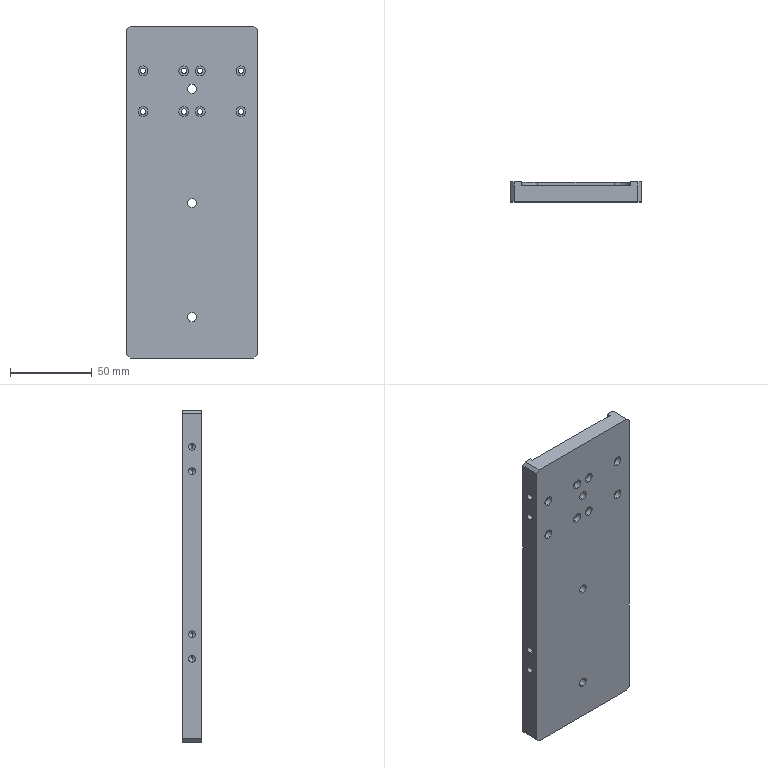Part | STEP file | PN_0022 | 1 solid | 119 faces | box 80 x 12 x 203.5 mm | volume 178921 mm3 | cylinder 70 | plane 25 | cone 24 | commonest cylinder face diameters 3.4 x16 4.2 x16 6 x16 5.5 x6 10 x6 4 x4